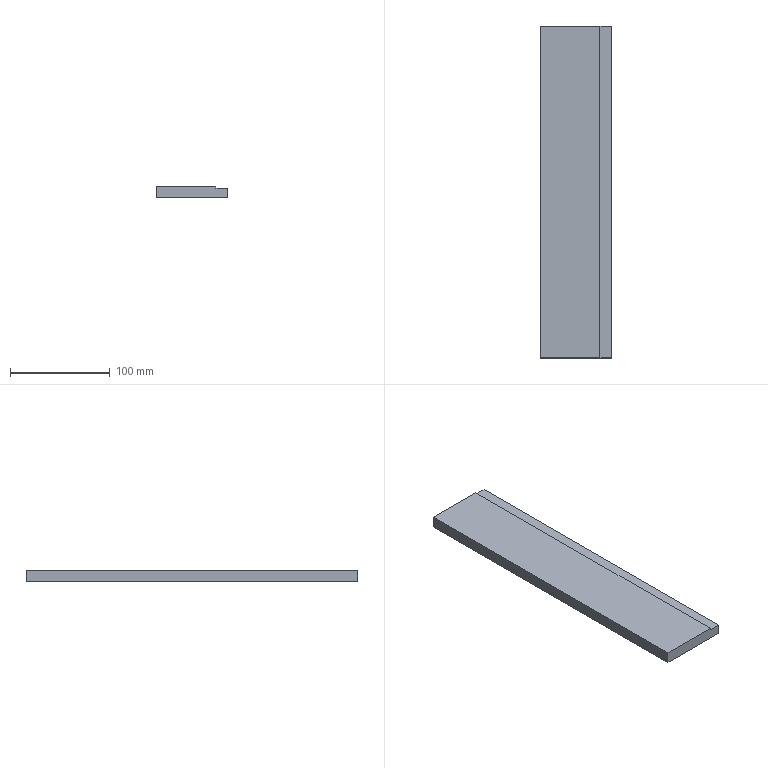Part | NX | features solid 2 | 1 solid | 8 faces | box 72 x 333 x 12 mm | volume 279720 mm3 | plane 8
STEP:
#1=CARTESIAN_POINT('',(-73.,443.3,54.866));
#2=VERTEX_POINT('',#1);
#3=CARTESIAN_POINT('',(-73.,110.3,54.866));
#4=VERTEX_POINT('',#3);
#5=CARTESIAN_POINT('',(-73.,145.3,54.866));
#6=DIRECTION('',(0.,-1.,0.));
#7=VECTOR('',#6,1000.);
#8=LINE('',#5,#7);
#9=EDGE_CURVE('',#2,#4,#8,.T.);
#10=ORIENTED_EDGE('',*,*,#9,.F.);
#11=CARTESIAN_POINT('',(-133.,443.3,54.866));
#12=VERTEX_POINT('',#11);
#13=CARTESIAN_POINT('',(-8.,443.3,54.866));
#14=DIRECTION('',(1.,0.,0.));
#15=VECTOR('',#14,1000.);
#16=LINE('',#13,#15);
#17=EDGE_CURVE('',#2,#12,#16,.F.);
#18=ORIENTED_EDGE('',*,*,#17,.T.);
#19=CARTESIAN_POINT('',(-133.,110.3,54.866));
#20=VERTEX_POINT('',#19);
#21=CARTESIAN_POINT('',(-133.,145.3,54.866));
#22=DIRECTION('',(0.,-1.,0.));
#23=VECTOR('',#22,1000.);
#24=LINE('',#21,#23);
#25=EDGE_CURVE('',#12,#20,#24,.T.);
#26=ORIENTED_EDGE('',*,*,#25,.T.);
#27=CARTESIAN_POINT('',(-8.,110.3,54.866));
#28=DIRECTION('',(1.,0.,0.));
#29=VECTOR('',#28,1000.);
#30=LINE('',#27,#29);
#31=EDGE_CURVE('',#4,#20,#30,.F.);
#32=ORIENTED_EDGE('',*,*,#31,.F.);
#33=EDGE_LOOP('',(#10,#18,#26,#32));
#34=FACE_BOUND('',#33,.T.);
#35=CARTESIAN_POINT('',(-8.,145.3,54.866));
#36=DIRECTION('',(0.,0.,1.));
#37=DIRECTION('',(-1.,0.,0.));
#38=AXIS2_PLACEMENT_3D('',#35,#36,#37);
#39=PLANE('',#38);
#40=ADVANCED_FACE('',(#34),#39,.T.);
#41=CARTESIAN_POINT('',(-61.,443.3,52.866));
#42=VERTEX_POINT('',#41);
#43=CARTESIAN_POINT('',(-61.,443.3,42.866));
#44=VERTEX_POINT('',#43);
#45=CARTESIAN_POINT('',(-61.,443.3,48.866));
#46=DIRECTION('',(0.,0.,-1.));
#47=VECTOR('',#46,1000.);
#48=LINE('',#45,#47);
#49=EDGE_CURVE('',#42,#44,#48,.T.);
#50=ORIENTED_EDGE('',*,*,#49,.F.);
#51=CARTESIAN_POINT('',(-61.,110.3,52.866));
#52=VERTEX_POINT('',#51);
#53=CARTESIAN_POINT('',(-61.,145.3,52.866));
#54=DIRECTION('',(0.,1.,0.));
#55=VECTOR('',#54,1000.);
#56=LINE('',#53,#55);
#57=EDGE_CURVE('',#42,#52,#56,.F.);
#58=ORIENTED_EDGE('',*,*,#57,.T.);
#59=CARTESIAN_POINT('',(-61.,110.3,42.866));
#60=VERTEX_POINT('',#59);
#61=CARTESIAN_POINT('',(-61.,110.3,48.866));
#62=DIRECTION('',(0.,0.,1.));
#63=VECTOR('',#62,1000.);
#64=LINE('',#61,#63);
#65=EDGE_CURVE('',#60,#52,#64,.T.);
#66=ORIENTED_EDGE('',*,*,#65,.F.);
#67=CARTESIAN_POINT('',(-61.,145.3,42.866));
#68=DIRECTION('',(0.,-1.,0.));
#69=VECTOR('',#68,1000.);
#70=LINE('',#67,#69);
#71=EDGE_CURVE('',#44,#60,#70,.T.);
#72=ORIENTED_EDGE('',*,*,#71,.F.);
#73=EDGE_LOOP('',(#50,#58,#66,#72));
#74=FACE_BOUND('',#73,.T.);
#75=CARTESIAN_POINT('',(-61.,145.3,84.));
#76=DIRECTION('',(1.,0.,0.));
#77=DIRECTION('',(0.,0.,-1.));
#78=AXIS2_PLACEMENT_3D('',#75,#76,#77);
#79=PLANE('',#78);
#80=ADVANCED_FACE('',(#74),#79,.T.);
#81=ORIENTED_EDGE('',*,*,#65,.T.);
#82=CARTESIAN_POINT('',(-73.,110.3,52.866));
#83=VERTEX_POINT('',#82);
#84=CARTESIAN_POINT('',(-67.,110.3,52.866));
#85=DIRECTION('',(1.,0.,0.));
#86=VECTOR('',#85,1000.);
#87=LINE('',#84,#86);
#88=EDGE_CURVE('',#83,#52,#87,.T.);
#89=ORIENTED_EDGE('',*,*,#88,.F.);
#90=CARTESIAN_POINT('',(-73.,110.3,107.866));
#91=DIRECTION('',(0.,0.,1.));
#92=VECTOR('',#91,1000.);
#93=LINE('',#90,#92);
#94=EDGE_CURVE('',#83,#4,#93,.T.);
#95=ORIENTED_EDGE('',*,*,#94,.T.);
#96=ORIENTED_EDGE('',*,*,#31,.T.);
#97=CARTESIAN_POINT('',(-133.,110.3,42.866));
#98=VERTEX_POINT('',#97);
#99=CARTESIAN_POINT('',(-133.,110.3,48.866));
#100=DIRECTION('',(0.,0.,-1.));
#101=VECTOR('',#100,1000.);
#102=LINE('',#99,#101);
#103=EDGE_CURVE('',#20,#98,#102,.T.);
#104=ORIENTED_EDGE('',*,*,#103,.T.);
#105=CARTESIAN_POINT('',(-8.,110.3,42.866));
#106=DIRECTION('',(1.,0.,0.));
#107=VECTOR('',#106,1000.);
#108=LINE('',#105,#107);
#109=EDGE_CURVE('',#60,#98,#108,.F.);
#110=ORIENTED_EDGE('',*,*,#109,.F.);
#111=EDGE_LOOP('',(#81,#89,#95,#96,#104,#110));
#112=FACE_BOUND('',#111,.T.);
#113=CARTESIAN_POINT('',(-8.,110.3,48.866));
#114=DIRECTION('',(0.,-1.,0.));
#115=DIRECTION('',(-1.,0.,0.));
#116=AXIS2_PLACEMENT_3D('',#113,#114,#115);
#117=PLANE('',#116);
#118=ADVANCED_FACE('',(#112),#117,.T.);
#119=ORIENTED_EDGE('',*,*,#109,.T.);
#120=CARTESIAN_POINT('',(-133.,443.3,42.866));
#121=VERTEX_POINT('',#120);
#122=CARTESIAN_POINT('',(-133.,145.3,42.866));
#123=DIRECTION('',(0.,1.,0.));
#124=VECTOR('',#123,1000.);
#125=LINE('',#122,#124);
#126=EDGE_CURVE('',#98,#121,#125,.T.);
#127=ORIENTED_EDGE('',*,*,#126,.T.);
#128=CARTESIAN_POINT('',(-8.,443.3,42.866));
#129=DIRECTION('',(1.,0.,0.));
#130=VECTOR('',#129,1000.);
#131=LINE('',#128,#130);
#132=EDGE_CURVE('',#44,#121,#131,.F.);
#133=ORIENTED_EDGE('',*,*,#132,.F.);
#134=ORIENTED_EDGE('',*,*,#71,.T.);
#135=EDGE_LOOP('',(#119,#127,#133,#134));
#136=FACE_BOUND('',#135,.T.);
#137=CARTESIAN_POINT('',(-8.,145.3,42.866));
#138=DIRECTION('',(0.,0.,-1.));
#139=DIRECTION('',(1.,0.,0.));
#140=AXIS2_PLACEMENT_3D('',#137,#138,#139);
#141=PLANE('',#140);
#142=ADVANCED_FACE('',(#136),#141,.T.);
#143=CARTESIAN_POINT('',(-73.,443.3,52.866));
#144=VERTEX_POINT('',#143);
#145=CARTESIAN_POINT('',(-73.,443.3,107.866));
#146=DIRECTION('',(0.,0.,1.));
#147=VECTOR('',#146,1000.);
#148=LINE('',#145,#147);
#149=EDGE_CURVE('',#144,#2,#148,.T.);
#150=ORIENTED_EDGE('',*,*,#149,.F.);
#151=CARTESIAN_POINT('',(-67.,443.3,52.866));
#152=DIRECTION('',(-1.,0.,0.));
#153=VECTOR('',#152,1000.);
#154=LINE('',#151,#153);
#155=EDGE_CURVE('',#42,#144,#154,.T.);
#156=ORIENTED_EDGE('',*,*,#155,.F.);
#157=ORIENTED_EDGE('',*,*,#49,.T.);
#158=ORIENTED_EDGE('',*,*,#132,.T.);
#159=CARTESIAN_POINT('',(-133.,443.3,48.866));
#160=DIRECTION('',(0.,0.,1.));
#161=VECTOR('',#160,1000.);
#162=LINE('',#159,#161);
#163=EDGE_CURVE('',#121,#12,#162,.T.);
#164=ORIENTED_EDGE('',*,*,#163,.T.);
#165=ORIENTED_EDGE('',*,*,#17,.F.);
#166=EDGE_LOOP('',(#150,#156,#157,#158,#164,#165));
#167=FACE_BOUND('',#166,.T.);
#168=CARTESIAN_POINT('',(-8.,443.3,48.866));
#169=DIRECTION('',(0.,1.,0.));
#170=DIRECTION('',(1.,0.,0.));
#171=AXIS2_PLACEMENT_3D('',#168,#169,#170);
#172=PLANE('',#171);
#173=ADVANCED_FACE('',(#167),#172,.T.);
#174=ORIENTED_EDGE('',*,*,#25,.F.);
#175=ORIENTED_EDGE('',*,*,#163,.F.);
#176=ORIENTED_EDGE('',*,*,#126,.F.);
#177=ORIENTED_EDGE('',*,*,#103,.F.);
#178=EDGE_LOOP('',(#174,#175,#176,#177));
#179=FACE_BOUND('',#178,.T.);
#180=CARTESIAN_POINT('',(-133.,145.3,48.866));
#181=DIRECTION('',(-1.,0.,0.));
#182=DIRECTION('',(0.,0.,-1.));
#183=AXIS2_PLACEMENT_3D('',#180,#181,#182);
#184=PLANE('',#183);
#185=ADVANCED_FACE('',(#179),#184,.T.);
#186=ORIENTED_EDGE('',*,*,#9,.T.);
#187=ORIENTED_EDGE('',*,*,#94,.F.);
#188=CARTESIAN_POINT('',(-73.,145.3,52.866));
#189=DIRECTION('',(0.,-1.,0.));
#190=VECTOR('',#189,1000.);
#191=LINE('',#188,#190);
#192=EDGE_CURVE('',#83,#144,#191,.F.);
#193=ORIENTED_EDGE('',*,*,#192,.T.);
#194=ORIENTED_EDGE('',*,*,#149,.T.);
#195=EDGE_LOOP('',(#186,#187,#193,#194));
#196=FACE_BOUND('',#195,.T.);
#197=CARTESIAN_POINT('',(-73.,145.3,107.866));
#198=DIRECTION('',(-1.,0.,0.));
#199=DIRECTION('',(0.,0.,1.));
#200=AXIS2_PLACEMENT_3D('',#197,#198,#199);
#201=PLANE('',#200);
#202=ADVANCED_FACE('',(#196),#201,.F.);
#203=ORIENTED_EDGE('',*,*,#57,.F.);
#204=ORIENTED_EDGE('',*,*,#155,.T.);
#205=ORIENTED_EDGE('',*,*,#192,.F.);
#206=ORIENTED_EDGE('',*,*,#88,.T.);
#207=EDGE_LOOP('',(#203,#204,#205,#206));
#208=FACE_BOUND('',#207,.T.);
#209=CARTESIAN_POINT('',(-67.,145.3,52.866));
#210=DIRECTION('',(0.,0.,-1.));
#211=DIRECTION('',(-1.,0.,0.));
#212=AXIS2_PLACEMENT_3D('',#209,#210,#211);
#213=PLANE('',#212);
#214=ADVANCED_FACE('',(#208),#213,.F.);
#215=CLOSED_SHELL('',(#40,#80,#118,#142,#173,#185,#202,#214));
#216=MANIFOLD_SOLID_BREP('',#215);
#217=(LENGTH_UNIT()NAMED_UNIT(*)SI_UNIT(.MILLI.,.METRE.));
#218=UNCERTAINTY_MEASURE_WITH_UNIT(LENGTH_MEASURE(0.00001),#217,'','');
#219=(NAMED_UNIT(*)PLANE_ANGLE_UNIT()SI_UNIT($,.RADIAN.));
#220=(NAMED_UNIT(*)SI_UNIT($,.STERADIAN.)SOLID_ANGLE_UNIT());
#221=(GEOMETRIC_REPRESENTATION_CONTEXT(3)GLOBAL_UNCERTAINTY_ASSIGNED_CONTEXT((#218))GLOBAL_UNIT_ASSIGNED_CONTEXT((#217,#219,#220))REPRESENTATION_CONTEXT('',''));
#222=ADVANCED_BREP_SHAPE_REPRESENTATION('',(#216),#221);